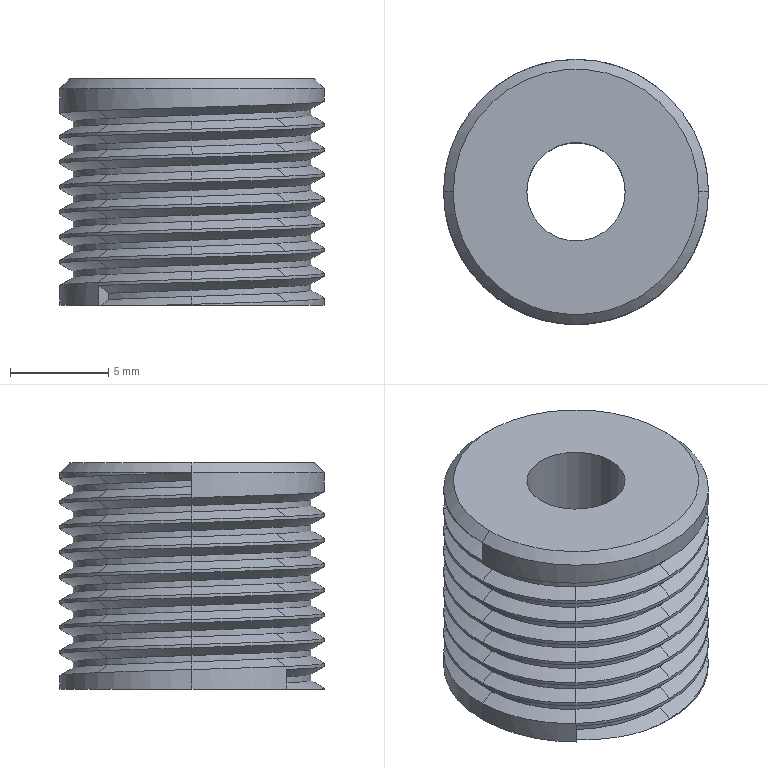Part | NX | features BREP 1 | 1 solid | 168 faces | box 13.458 x 13.458 x 11.5 mm | volume 1248 mm3 | spline 126 | cylinder 36 | plane 4 | cone 2 | commonest cylinder face diameters 13.458 x18 12.083 x16 5 x2